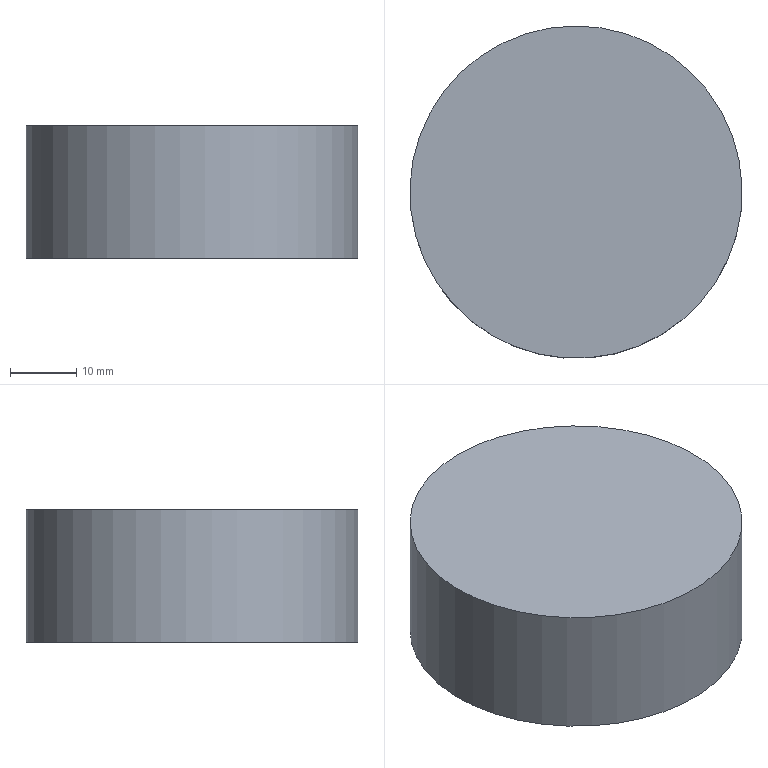Part | NX | features solid 2 | 1 solid | 3 faces | box 50 x 50 x 20 mm | volume 39270 mm3 | plane 2 | cylinder 1 | commonest cylinder face diameters 50 x1
STEP:
#1=CARTESIAN_POINT('',(-130.456,170.697,70.));
#2=VERTEX_POINT('',#1);
#3=CARTESIAN_POINT('',(-144.796,150.218,70.));
#4=DIRECTION('',(0.,0.,1.));
#5=DIRECTION('',(0.5736,0.8192,0.));
#6=AXIS2_PLACEMENT_3D('',#3,#4,#5);
#7=CIRCLE('',#6,25.);
#8=EDGE_CURVE('',#2,#2,#7,.T.);
#9=ORIENTED_EDGE('',*,*,#8,.T.);
#10=EDGE_LOOP('',(#9));
#11=FACE_BOUND('',#10,.T.);
#12=CARTESIAN_POINT('',(-130.456,170.697,90.));
#13=VERTEX_POINT('',#12);
#14=CARTESIAN_POINT('',(-144.796,150.218,90.));
#15=DIRECTION('',(0.,0.,1.));
#16=DIRECTION('',(0.5736,0.8192,0.));
#17=AXIS2_PLACEMENT_3D('',#14,#15,#16);
#18=CIRCLE('',#17,25.);
#19=EDGE_CURVE('',#13,#13,#18,.T.);
#20=ORIENTED_EDGE('',*,*,#19,.F.);
#21=EDGE_LOOP('',(#20));
#22=FACE_BOUND('',#21,.T.);
#23=CARTESIAN_POINT('',(-144.796,150.218,70.));
#24=DIRECTION('',(0.,0.,1.));
#25=DIRECTION('',(1.,0.,0.));
#26=AXIS2_PLACEMENT_3D('',#23,#24,#25);
#27=CYLINDRICAL_SURFACE('',#26,25.);
#28=ADVANCED_FACE('',(#11,#22),#27,.T.);
#29=ORIENTED_EDGE('',*,*,#8,.F.);
#30=EDGE_LOOP('',(#29));
#31=FACE_BOUND('',#30,.T.);
#32=CARTESIAN_POINT('',(-144.796,150.218,70.));
#33=DIRECTION('',(0.,0.,1.));
#34=DIRECTION('',(1.,0.,0.));
#35=AXIS2_PLACEMENT_3D('',#32,#33,#34);
#36=PLANE('',#35);
#37=ADVANCED_FACE('',(#31),#36,.F.);
#38=ORIENTED_EDGE('',*,*,#19,.T.);
#39=EDGE_LOOP('',(#38));
#40=FACE_BOUND('',#39,.T.);
#41=CARTESIAN_POINT('',(-144.796,150.218,90.));
#42=DIRECTION('',(0.,0.,1.));
#43=DIRECTION('',(1.,0.,0.));
#44=AXIS2_PLACEMENT_3D('',#41,#42,#43);
#45=PLANE('',#44);
#46=ADVANCED_FACE('',(#40),#45,.T.);
#47=CLOSED_SHELL('',(#28,#37,#46));
#48=MANIFOLD_SOLID_BREP('',#47);
#49=(LENGTH_UNIT()NAMED_UNIT(*)SI_UNIT(.MILLI.,.METRE.));
#50=UNCERTAINTY_MEASURE_WITH_UNIT(LENGTH_MEASURE(0.00001),#49,'','');
#51=(NAMED_UNIT(*)PLANE_ANGLE_UNIT()SI_UNIT($,.RADIAN.));
#52=(NAMED_UNIT(*)SI_UNIT($,.STERADIAN.)SOLID_ANGLE_UNIT());
#53=(GEOMETRIC_REPRESENTATION_CONTEXT(3)GLOBAL_UNCERTAINTY_ASSIGNED_CONTEXT((#50))GLOBAL_UNIT_ASSIGNED_CONTEXT((#49,#51,#52))REPRESENTATION_CONTEXT('',''));
#54=ADVANCED_BREP_SHAPE_REPRESENTATION('',(#48),#53);